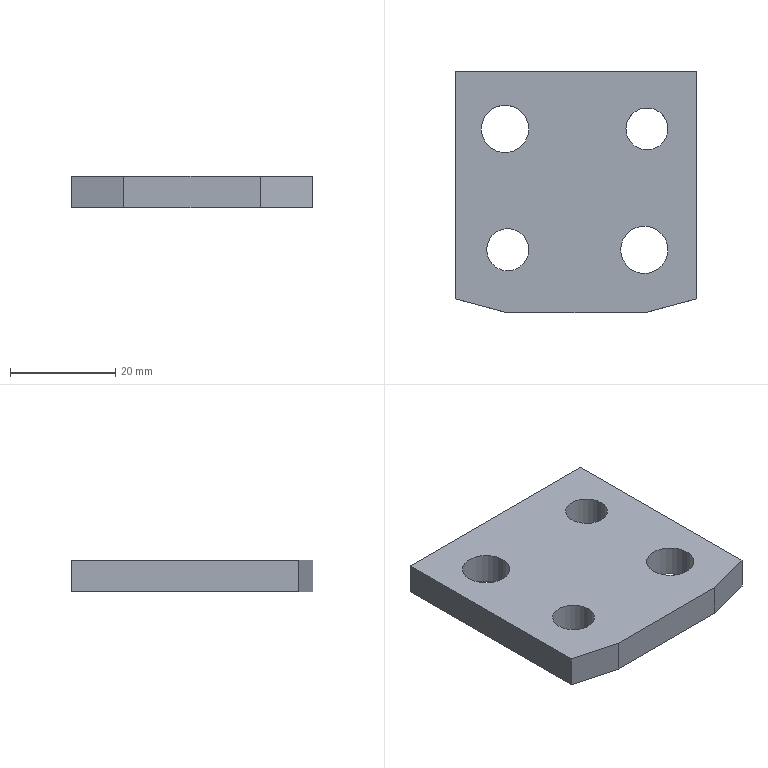Part | STEP file | gslz 2016.10.28-13_id682_x_t | 1 solid | 12 faces | box 46 x 46 x 6 mm | volume 11169 mm3 | plane 8 | cylinder 4 | commonest cylinder face diameters 8 x2 9 x2
STEP:
#1=CARTESIAN_POINT('',(0.,0.,0.));
#2=DIRECTION('',(0.,0.,1.));
#3=DIRECTION('',(1.,0.,0.));
#4=AXIS2_PLACEMENT_3D('',#1,#2,#3);
#5=CARTESIAN_POINT('',(1187.998,279.75,6.));
#6=VERTEX_POINT('',#5);
#7=CARTESIAN_POINT('',(1179.998,279.75,6.));
#8=VERTEX_POINT('',#7);
#9=CARTESIAN_POINT('',(1183.998,279.75,6.));
#10=DIRECTION('',(0.,0.,1.));
#11=DIRECTION('',(-1.,0.,0.));
#12=AXIS2_PLACEMENT_3D('',#9,#10,#11);
#13=CIRCLE('',#12,4.);
#14=CARTESIAN_POINT('',(1183.998,279.75,-73.));
#15=DIRECTION('',(0.,0.,1.));
#16=DIRECTION('',(1.,0.,0.));
#17=AXIS2_PLACEMENT_3D('',#14,#15,#16);
#18=CYLINDRICAL_SURFACE('',#17,4.);
#19=CARTESIAN_POINT('',(-3.142,79.));
#20=DIRECTION('',(1.,0.));
#21=VECTOR('',#20,1.);
#22=LINE('',#19,#21);
#23=(GEOMETRIC_REPRESENTATION_CONTEXT(2)PARAMETRIC_REPRESENTATION_CONTEXT()REPRESENTATION_CONTEXT('',''));
#24=DEFINITIONAL_REPRESENTATION('',(#22),#23);
#25=PCURVE('',#18,#24);
#26=CARTESIAN_POINT('',(1116.998,263.25,6.));
#27=DIRECTION('',(0.,0.,-1.));
#28=DIRECTION('',(-1.,0.,0.));
#29=AXIS2_PLACEMENT_3D('',#26,#27,#28);
#30=PLANE('',#29);
#31=CARTESIAN_POINT('',(-63.,16.5));
#32=CARTESIAN_POINT('',(-63.,9.572));
#33=CARTESIAN_POINT('',(-69.,13.036));
#34=CARTESIAN_POINT('',(-75.,16.5));
#35=CARTESIAN_POINT('',(-69.,19.964));
#36=CARTESIAN_POINT('',(-63.,23.428));
#37=CARTESIAN_POINT('',(-63.,16.5));
#38=(BOUNDED_CURVE()B_SPLINE_CURVE(2,(#31,#32,#33,#34,#35,#36,#37),.UNSPECIFIED.,.T.,.F.)B_SPLINE_CURVE_WITH_KNOTS((1,2,2,2,2,1),(-2.094,0.,2.094,4.189,6.283,8.378),.UNSPECIFIED.)CURVE()GEOMETRIC_REPRESENTATION_ITEM()RATIONAL_B_SPLINE_CURVE((1.,0.5,1.,0.5,1.,0.5,1.))REPRESENTATION_ITEM(''));
#39=(GEOMETRIC_REPRESENTATION_CONTEXT(2)PARAMETRIC_REPRESENTATION_CONTEXT()REPRESENTATION_CONTEXT('',''));
#40=DEFINITIONAL_REPRESENTATION('',(#38),#39);
#41=PCURVE('',#30,#40);
#42=SURFACE_CURVE('',#13,(#25,#41),.PCURVE_S1.);
#43=EDGE_CURVE('',#6,#8,#42,.T.);
#44=ORIENTED_EDGE('',*,*,#43,.F.);
#45=CARTESIAN_POINT('',(1187.998,279.75,0.));
#46=VERTEX_POINT('',#45);
#47=CARTESIAN_POINT('',(1187.998,279.75,0.));
#48=CARTESIAN_POINT('',(1187.998,279.75,6.));
#49=B_SPLINE_CURVE_WITH_KNOTS('',1,(#47,#48),.UNSPECIFIED.,.F.,.F.,(2,2),(73.,79.),.PIECEWISE_BEZIER_KNOTS.);
#50=CARTESIAN_POINT('',(0.,0.));
#51=DIRECTION('',(0.,1.));
#52=VECTOR('',#51,1.);
#53=LINE('',#50,#52);
#54=(GEOMETRIC_REPRESENTATION_CONTEXT(2)PARAMETRIC_REPRESENTATION_CONTEXT()REPRESENTATION_CONTEXT('',''));
#55=DEFINITIONAL_REPRESENTATION('',(#53),#54);
#56=PCURVE('',#18,#55);
#57=CARTESIAN_POINT('',(6.283,0.));
#58=DIRECTION('',(0.,1.));
#59=VECTOR('',#58,1.);
#60=LINE('',#57,#59);
#61=(GEOMETRIC_REPRESENTATION_CONTEXT(2)PARAMETRIC_REPRESENTATION_CONTEXT()REPRESENTATION_CONTEXT('',''));
#62=DEFINITIONAL_REPRESENTATION('',(#60),#61);
#63=PCURVE('',#18,#62);
#64=SEAM_CURVE('',#49,(#56,#63),.PCURVE_S1.);
#65=EDGE_CURVE('',#46,#6,#64,.T.);
#66=ORIENTED_EDGE('',*,*,#65,.F.);
#67=CARTESIAN_POINT('',(1183.998,279.75,0.));
#68=DIRECTION('',(0.,0.,-1.));
#69=DIRECTION('',(1.,0.,0.));
#70=AXIS2_PLACEMENT_3D('',#67,#68,#69);
#71=CIRCLE('',#70,4.);
#72=CARTESIAN_POINT('',(6.283,73.));
#73=DIRECTION('',(-1.,0.));
#74=VECTOR('',#73,1.);
#75=LINE('',#72,#74);
#76=(GEOMETRIC_REPRESENTATION_CONTEXT(2)PARAMETRIC_REPRESENTATION_CONTEXT()REPRESENTATION_CONTEXT('',''));
#77=DEFINITIONAL_REPRESENTATION('',(#75),#76);
#78=PCURVE('',#18,#77);
#79=CARTESIAN_POINT('',(1076.998,293.75,0.));
#80=DIRECTION('',(0.,0.,1.));
#81=DIRECTION('',(1.,0.,0.));
#82=AXIS2_PLACEMENT_3D('',#79,#80,#81);
#83=PLANE('',#82);
#84=CARTESIAN_POINT('',(111.,-14.));
#85=CARTESIAN_POINT('',(111.,-20.928));
#86=CARTESIAN_POINT('',(105.,-17.464));
#87=CARTESIAN_POINT('',(99.,-14.));
#88=CARTESIAN_POINT('',(105.,-10.536));
#89=CARTESIAN_POINT('',(111.,-7.072));
#90=CARTESIAN_POINT('',(111.,-14.));
#91=(BOUNDED_CURVE()B_SPLINE_CURVE(2,(#84,#85,#86,#87,#88,#89,#90),.UNSPECIFIED.,.T.,.F.)B_SPLINE_CURVE_WITH_KNOTS((1,2,2,2,2,1),(-2.094,0.,2.094,4.189,6.283,8.378),.UNSPECIFIED.)CURVE()GEOMETRIC_REPRESENTATION_ITEM()RATIONAL_B_SPLINE_CURVE((1.,0.5,1.,0.5,1.,0.5,1.))REPRESENTATION_ITEM(''));
#92=(GEOMETRIC_REPRESENTATION_CONTEXT(2)PARAMETRIC_REPRESENTATION_CONTEXT()REPRESENTATION_CONTEXT('',''));
#93=DEFINITIONAL_REPRESENTATION('',(#91),#92);
#94=PCURVE('',#83,#93);
#95=SURFACE_CURVE('',#71,(#78,#94),.PCURVE_S1.);
#96=EDGE_CURVE('',#46,#46,#95,.T.);
#97=ORIENTED_EDGE('',*,*,#96,.F.);
#98=ORIENTED_EDGE('',*,*,#65,.T.);
#99=CARTESIAN_POINT('',(1183.998,279.75,6.));
#100=DIRECTION('',(0.,0.,1.));
#101=DIRECTION('',(-1.,0.,0.));
#102=AXIS2_PLACEMENT_3D('',#99,#100,#101);
#103=CIRCLE('',#102,4.);
#104=CARTESIAN_POINT('',(3.142,79.));
#105=DIRECTION('',(1.,0.));
#106=VECTOR('',#105,1.);
#107=LINE('',#104,#106);
#108=(GEOMETRIC_REPRESENTATION_CONTEXT(2)PARAMETRIC_REPRESENTATION_CONTEXT()REPRESENTATION_CONTEXT('',''));
#109=DEFINITIONAL_REPRESENTATION('',(#107),#108);
#110=PCURVE('',#18,#109);
#111=CARTESIAN_POINT('',(-63.,16.5));
#112=CARTESIAN_POINT('',(-63.,9.572));
#113=CARTESIAN_POINT('',(-69.,13.036));
#114=CARTESIAN_POINT('',(-75.,16.5));
#115=CARTESIAN_POINT('',(-69.,19.964));
#116=CARTESIAN_POINT('',(-63.,23.428));
#117=CARTESIAN_POINT('',(-63.,16.5));
#118=(BOUNDED_CURVE()B_SPLINE_CURVE(2,(#111,#112,#113,#114,#115,#116,#117),.UNSPECIFIED.,.T.,.F.)B_SPLINE_CURVE_WITH_KNOTS((1,2,2,2,2,1),(-2.094,0.,2.094,4.189,6.283,8.378),.UNSPECIFIED.)CURVE()GEOMETRIC_REPRESENTATION_ITEM()RATIONAL_B_SPLINE_CURVE((1.,0.5,1.,0.5,1.,0.5,1.))REPRESENTATION_ITEM(''));
#119=(GEOMETRIC_REPRESENTATION_CONTEXT(2)PARAMETRIC_REPRESENTATION_CONTEXT()REPRESENTATION_CONTEXT('',''));
#120=DEFINITIONAL_REPRESENTATION('',(#118),#119);
#121=PCURVE('',#30,#120);
#122=SURFACE_CURVE('',#103,(#110,#121),.PCURVE_S1.);
#123=EDGE_CURVE('',#8,#6,#122,.T.);
#124=ORIENTED_EDGE('',*,*,#123,.F.);
#125=EDGE_LOOP('',(#44,#66,#97,#98,#124));
#126=FACE_BOUND('',#125,.F.);
#127=ADVANCED_FACE('',(#126),#18,.F.);
#128=CARTESIAN_POINT('',(1205.498,279.75,6.));
#129=VERTEX_POINT('',#128);
#130=CARTESIAN_POINT('',(1214.498,279.75,6.));
#131=VERTEX_POINT('',#130);
#132=CARTESIAN_POINT('',(1209.998,279.75,6.));
#133=DIRECTION('',(0.,0.,-1.));
#134=DIRECTION('',(-1.,0.,0.));
#135=AXIS2_PLACEMENT_3D('',#132,#133,#134);
#136=CIRCLE('',#135,4.5);
#137=CARTESIAN_POINT('',(1209.998,279.75,-73.));
#138=DIRECTION('',(0.,0.,1.));
#139=DIRECTION('',(1.,0.,0.));
#140=AXIS2_PLACEMENT_3D('',#137,#138,#139);
#141=CYLINDRICAL_SURFACE('',#140,4.5);
#142=CARTESIAN_POINT('',(3.142,79.));
#143=DIRECTION('',(-1.,0.));
#144=VECTOR('',#143,1.);
#145=LINE('',#142,#144);
#146=(GEOMETRIC_REPRESENTATION_CONTEXT(2)PARAMETRIC_REPRESENTATION_CONTEXT()REPRESENTATION_CONTEXT('',''));
#147=DEFINITIONAL_REPRESENTATION('',(#145),#146);
#148=PCURVE('',#141,#147);
#149=CARTESIAN_POINT('',(-93.,16.5));
#150=DIRECTION('',(1.,0.));
#151=AXIS2_PLACEMENT_2D('',#149,#150);
#152=CIRCLE('',#151,4.5);
#153=(GEOMETRIC_REPRESENTATION_CONTEXT(2)PARAMETRIC_REPRESENTATION_CONTEXT()REPRESENTATION_CONTEXT('',''));
#154=DEFINITIONAL_REPRESENTATION('',(#152),#153);
#155=PCURVE('',#30,#154);
#156=SURFACE_CURVE('',#136,(#148,#155),.PCURVE_S1.);
#157=EDGE_CURVE('',#129,#131,#156,.T.);
#158=ORIENTED_EDGE('',*,*,#157,.T.);
#159=CARTESIAN_POINT('',(1214.498,279.75,0.));
#160=VERTEX_POINT('',#159);
#161=CARTESIAN_POINT('',(1214.498,279.75,0.));
#162=CARTESIAN_POINT('',(1214.498,279.75,6.));
#163=B_SPLINE_CURVE_WITH_KNOTS('',1,(#161,#162),.UNSPECIFIED.,.F.,.F.,(2,2),(73.,79.),.PIECEWISE_BEZIER_KNOTS.);
#164=CARTESIAN_POINT('',(0.,0.));
#165=DIRECTION('',(0.,1.));
#166=VECTOR('',#165,1.);
#167=LINE('',#164,#166);
#168=(GEOMETRIC_REPRESENTATION_CONTEXT(2)PARAMETRIC_REPRESENTATION_CONTEXT()REPRESENTATION_CONTEXT('',''));
#169=DEFINITIONAL_REPRESENTATION('',(#167),#168);
#170=PCURVE('',#141,#169);
#171=CARTESIAN_POINT('',(6.283,0.));
#172=DIRECTION('',(0.,1.));
#173=VECTOR('',#172,1.);
#174=LINE('',#171,#173);
#175=(GEOMETRIC_REPRESENTATION_CONTEXT(2)PARAMETRIC_REPRESENTATION_CONTEXT()REPRESENTATION_CONTEXT('',''));
#176=DEFINITIONAL_REPRESENTATION('',(#174),#175);
#177=PCURVE('',#141,#176);
#178=SEAM_CURVE('',#163,(#170,#177),.PCURVE_S1.);
#179=EDGE_CURVE('',#160,#131,#178,.T.);
#180=ORIENTED_EDGE('',*,*,#179,.F.);
#181=CARTESIAN_POINT('',(1209.998,279.75,0.));
#182=DIRECTION('',(0.,0.,1.));
#183=DIRECTION('',(1.,0.,0.));
#184=AXIS2_PLACEMENT_3D('',#181,#182,#183);
#185=CIRCLE('',#184,4.5);
#186=CARTESIAN_POINT('',(0.,73.));
#187=DIRECTION('',(1.,0.));
#188=VECTOR('',#187,1.);
#189=LINE('',#186,#188);
#190=(GEOMETRIC_REPRESENTATION_CONTEXT(2)PARAMETRIC_REPRESENTATION_CONTEXT()REPRESENTATION_CONTEXT('',''));
#191=DEFINITIONAL_REPRESENTATION('',(#189),#190);
#192=PCURVE('',#141,#191);
#193=CARTESIAN_POINT('',(133.,-14.));
#194=DIRECTION('',(1.,0.));
#195=AXIS2_PLACEMENT_2D('',#193,#194);
#196=CIRCLE('',#195,4.5);
#197=(GEOMETRIC_REPRESENTATION_CONTEXT(2)PARAMETRIC_REPRESENTATION_CONTEXT()REPRESENTATION_CONTEXT('',''));
#198=DEFINITIONAL_REPRESENTATION('',(#196),#197);
#199=PCURVE('',#83,#198);
#200=SURFACE_CURVE('',#185,(#192,#199),.PCURVE_S1.);
#201=EDGE_CURVE('',#160,#160,#200,.T.);
#202=ORIENTED_EDGE('',*,*,#201,.T.);
#203=ORIENTED_EDGE('',*,*,#179,.T.);
#204=CARTESIAN_POINT('',(1209.998,279.75,6.));
#205=DIRECTION('',(0.,0.,-1.));
#206=DIRECTION('',(-1.,0.,0.));
#207=AXIS2_PLACEMENT_3D('',#204,#205,#206);
#208=CIRCLE('',#207,4.5);
#209=CARTESIAN_POINT('',(9.425,79.));
#210=DIRECTION('',(-1.,0.));
#211=VECTOR('',#210,1.);
#212=LINE('',#209,#211);
#213=(GEOMETRIC_REPRESENTATION_CONTEXT(2)PARAMETRIC_REPRESENTATION_CONTEXT()REPRESENTATION_CONTEXT('',''));
#214=DEFINITIONAL_REPRESENTATION('',(#212),#213);
#215=PCURVE('',#141,#214);
#216=CARTESIAN_POINT('',(-93.,16.5));
#217=DIRECTION('',(1.,0.));
#218=AXIS2_PLACEMENT_2D('',#216,#217);
#219=CIRCLE('',#218,4.5);
#220=(GEOMETRIC_REPRESENTATION_CONTEXT(2)PARAMETRIC_REPRESENTATION_CONTEXT()REPRESENTATION_CONTEXT('',''));
#221=DEFINITIONAL_REPRESENTATION('',(#219),#220);
#222=PCURVE('',#30,#221);
#223=SURFACE_CURVE('',#208,(#215,#222),.PCURVE_S1.);
#224=EDGE_CURVE('',#131,#129,#223,.T.);
#225=ORIENTED_EDGE('',*,*,#224,.T.);
#226=EDGE_LOOP('',(#158,#180,#202,#203,#225));
#227=FACE_BOUND('',#226,.F.);
#228=ADVANCED_FACE('',(#227),#141,.F.);
#229=CARTESIAN_POINT('',(1178.998,302.75,6.));
#230=VERTEX_POINT('',#229);
#231=CARTESIAN_POINT('',(1183.498,302.75,6.));
#232=DIRECTION('',(0.,0.,-1.));
#233=DIRECTION('',(-1.,0.,0.));
#234=AXIS2_PLACEMENT_3D('',#231,#232,#233);
#235=CIRCLE('',#234,4.5);
#236=CARTESIAN_POINT('',(1183.498,302.75,47.));
#237=DIRECTION('',(0.,0.,-1.));
#238=DIRECTION('',(-1.,0.,0.));
#239=AXIS2_PLACEMENT_3D('',#236,#237,#238);
#240=CYLINDRICAL_SURFACE('',#239,4.5);
#241=CARTESIAN_POINT('',(0.,41.));
#242=DIRECTION('',(1.,0.));
#243=VECTOR('',#242,1.);
#244=LINE('',#241,#243);
#245=(GEOMETRIC_REPRESENTATION_CONTEXT(2)PARAMETRIC_REPRESENTATION_CONTEXT()REPRESENTATION_CONTEXT('',''));
#246=DEFINITIONAL_REPRESENTATION('',(#244),#245);
#247=PCURVE('',#240,#246);
#248=CARTESIAN_POINT('',(-66.5,39.5));
#249=DIRECTION('',(1.,0.));
#250=AXIS2_PLACEMENT_2D('',#248,#249);
#251=CIRCLE('',#250,4.5);
#252=(GEOMETRIC_REPRESENTATION_CONTEXT(2)PARAMETRIC_REPRESENTATION_CONTEXT()REPRESENTATION_CONTEXT('',''));
#253=DEFINITIONAL_REPRESENTATION('',(#251),#252);
#254=PCURVE('',#30,#253);
#255=SURFACE_CURVE('',#235,(#247,#254),.PCURVE_S1.);
#256=EDGE_CURVE('',#230,#230,#255,.T.);
#257=ORIENTED_EDGE('',*,*,#256,.T.);
#258=CARTESIAN_POINT('',(1178.998,302.75,0.));
#259=VERTEX_POINT('',#258);
#260=CARTESIAN_POINT('',(1178.998,302.75,6.));
#261=CARTESIAN_POINT('',(1178.998,302.75,0.));
#262=B_SPLINE_CURVE_WITH_KNOTS('',1,(#260,#261),.UNSPECIFIED.,.F.,.F.,(2,2),(41.,47.),.PIECEWISE_BEZIER_KNOTS.);
#263=CARTESIAN_POINT('',(6.283,0.));
#264=DIRECTION('',(0.,1.));
#265=VECTOR('',#264,1.);
#266=LINE('',#263,#265);
#267=(GEOMETRIC_REPRESENTATION_CONTEXT(2)PARAMETRIC_REPRESENTATION_CONTEXT()REPRESENTATION_CONTEXT('',''));
#268=DEFINITIONAL_REPRESENTATION('',(#266),#267);
#269=PCURVE('',#240,#268);
#270=CARTESIAN_POINT('',(0.,0.));
#271=DIRECTION('',(0.,1.));
#272=VECTOR('',#271,1.);
#273=LINE('',#270,#272);
#274=(GEOMETRIC_REPRESENTATION_CONTEXT(2)PARAMETRIC_REPRESENTATION_CONTEXT()REPRESENTATION_CONTEXT('',''));
#275=DEFINITIONAL_REPRESENTATION('',(#273),#274);
#276=PCURVE('',#240,#275);
#277=SEAM_CURVE('',#262,(#269,#276),.PCURVE_S1.);
#278=EDGE_CURVE('',#230,#259,#277,.T.);
#279=ORIENTED_EDGE('',*,*,#278,.T.);
#280=CARTESIAN_POINT('',(1187.998,302.75,0.));
#281=VERTEX_POINT('',#280);
#282=CARTESIAN_POINT('',(1183.498,302.75,0.));
#283=DIRECTION('',(0.,0.,1.));
#284=DIRECTION('',(1.,0.,0.));
#285=AXIS2_PLACEMENT_3D('',#282,#283,#284);
#286=CIRCLE('',#285,4.5);
#287=CARTESIAN_POINT('',(9.425,47.));
#288=DIRECTION('',(-1.,0.));
#289=VECTOR('',#288,1.);
#290=LINE('',#287,#289);
#291=(GEOMETRIC_REPRESENTATION_CONTEXT(2)PARAMETRIC_REPRESENTATION_CONTEXT()REPRESENTATION_CONTEXT('',''));
#292=DEFINITIONAL_REPRESENTATION('',(#290),#291);
#293=PCURVE('',#240,#292);
#294=CARTESIAN_POINT('',(106.5,9.));
#295=DIRECTION('',(1.,0.));
#296=AXIS2_PLACEMENT_2D('',#294,#295);
#297=CIRCLE('',#296,4.5);
#298=(GEOMETRIC_REPRESENTATION_CONTEXT(2)PARAMETRIC_REPRESENTATION_CONTEXT()REPRESENTATION_CONTEXT('',''));
#299=DEFINITIONAL_REPRESENTATION('',(#297),#298);
#300=PCURVE('',#83,#299);
#301=SURFACE_CURVE('',#286,(#293,#300),.PCURVE_S1.);
#302=EDGE_CURVE('',#259,#281,#301,.T.);
#303=ORIENTED_EDGE('',*,*,#302,.T.);
#304=CARTESIAN_POINT('',(1183.498,302.75,0.));
#305=DIRECTION('',(0.,0.,1.));
#306=DIRECTION('',(1.,0.,0.));
#307=AXIS2_PLACEMENT_3D('',#304,#305,#306);
#308=CIRCLE('',#307,4.5);
#309=CARTESIAN_POINT('',(3.142,47.));
#310=DIRECTION('',(-1.,0.));
#311=VECTOR('',#310,1.);
#312=LINE('',#309,#311);
#313=(GEOMETRIC_REPRESENTATION_CONTEXT(2)PARAMETRIC_REPRESENTATION_CONTEXT()REPRESENTATION_CONTEXT('',''));
#314=DEFINITIONAL_REPRESENTATION('',(#312),#313);
#315=PCURVE('',#240,#314);
#316=CARTESIAN_POINT('',(106.5,9.));
#317=DIRECTION('',(1.,0.));
#318=AXIS2_PLACEMENT_2D('',#316,#317);
#319=CIRCLE('',#318,4.5);
#320=(GEOMETRIC_REPRESENTATION_CONTEXT(2)PARAMETRIC_REPRESENTATION_CONTEXT()REPRESENTATION_CONTEXT('',''));
#321=DEFINITIONAL_REPRESENTATION('',(#319),#320);
#322=PCURVE('',#83,#321);
#323=SURFACE_CURVE('',#308,(#315,#322),.PCURVE_S1.);
#324=EDGE_CURVE('',#281,#259,#323,.T.);
#325=ORIENTED_EDGE('',*,*,#324,.T.);
#326=ORIENTED_EDGE('',*,*,#278,.F.);
#327=EDGE_LOOP('',(#257,#279,#303,#325,#326));
#328=FACE_BOUND('',#327,.F.);
#329=ADVANCED_FACE('',(#328),#240,.F.);
#330=CARTESIAN_POINT('',(1209.999,267.75,0.));
#331=VERTEX_POINT('',#330);
#332=CARTESIAN_POINT('',(1209.999,267.75,6.));
#333=VERTEX_POINT('',#332);
#334=CARTESIAN_POINT('',(1209.999,267.75,8.));
#335=DIRECTION('',(0.,0.,1.));
#336=VECTOR('',#335,1.);
#337=LINE('',#334,#336);
#338=CARTESIAN_POINT('',(1087.,267.75,8.));
#339=DIRECTION('',(0.,1.,0.));
#340=DIRECTION('',(0.,0.,1.));
#341=AXIS2_PLACEMENT_3D('',#338,#339,#340);
#342=PLANE('',#341);
#343=CARTESIAN_POINT('',(0.,122.999));
#344=DIRECTION('',(1.,0.));
#345=VECTOR('',#344,1.);
#346=LINE('',#343,#345);
#347=(GEOMETRIC_REPRESENTATION_CONTEXT(2)PARAMETRIC_REPRESENTATION_CONTEXT()REPRESENTATION_CONTEXT('',''));
#348=DEFINITIONAL_REPRESENTATION('',(#346),#347);
#349=PCURVE('',#342,#348);
#350=CARTESIAN_POINT('',(1209.999,267.75,8.));
#351=DIRECTION('',(-0.2588,0.9659,0.));
#352=DIRECTION('',(-0.9659,-0.2588,0.));
#353=AXIS2_PLACEMENT_3D('',#350,#351,#352);
#354=PLANE('',#353);
#355=CARTESIAN_POINT('',(0.,0.));
#356=DIRECTION('',(0.,1.));
#357=VECTOR('',#356,1.);
#358=LINE('',#355,#357);
#359=(GEOMETRIC_REPRESENTATION_CONTEXT(2)PARAMETRIC_REPRESENTATION_CONTEXT()REPRESENTATION_CONTEXT('',''));
#360=DEFINITIONAL_REPRESENTATION('',(#358),#359);
#361=PCURVE('',#354,#360);
#362=SURFACE_CURVE('',#337,(#349,#361),.PCURVE_S1.);
#363=EDGE_CURVE('',#331,#333,#362,.T.);
#364=ORIENTED_EDGE('',*,*,#363,.T.);
#365=CARTESIAN_POINT('',(1184.,267.75,6.));
#366=VERTEX_POINT('',#365);
#367=CARTESIAN_POINT('',(1087.,267.75,6.));
#368=DIRECTION('',(-1.,0.,0.));
#369=VECTOR('',#368,1.);
#370=LINE('',#367,#369);
#371=CARTESIAN_POINT('',(-2.,0.));
#372=DIRECTION('',(0.,-1.));
#373=VECTOR('',#372,1.);
#374=LINE('',#371,#373);
#375=(GEOMETRIC_REPRESENTATION_CONTEXT(2)PARAMETRIC_REPRESENTATION_CONTEXT()REPRESENTATION_CONTEXT('',''));
#376=DEFINITIONAL_REPRESENTATION('',(#374),#375);
#377=PCURVE('',#342,#376);
#378=CARTESIAN_POINT('',(29.998,4.5));
#379=DIRECTION('',(1.,0.));
#380=VECTOR('',#379,1.);
#381=LINE('',#378,#380);
#382=(GEOMETRIC_REPRESENTATION_CONTEXT(2)PARAMETRIC_REPRESENTATION_CONTEXT()REPRESENTATION_CONTEXT('',''));
#383=DEFINITIONAL_REPRESENTATION('',(#381),#382);
#384=PCURVE('',#30,#383);
#385=SURFACE_CURVE('',#370,(#377,#384),.PCURVE_S1.);
#386=EDGE_CURVE('',#333,#366,#385,.T.);
#387=ORIENTED_EDGE('',*,*,#386,.T.);
#388=CARTESIAN_POINT('',(1184.,267.75,0.));
#389=VERTEX_POINT('',#388);
#390=CARTESIAN_POINT('',(1184.,267.75,8.));
#391=DIRECTION('',(0.,0.,1.));
#392=VECTOR('',#391,1.);
#393=LINE('',#390,#392);
#394=CARTESIAN_POINT('',(0.,97.));
#395=DIRECTION('',(1.,0.));
#396=VECTOR('',#395,1.);
#397=LINE('',#394,#396);
#398=(GEOMETRIC_REPRESENTATION_CONTEXT(2)PARAMETRIC_REPRESENTATION_CONTEXT()REPRESENTATION_CONTEXT('',''));
#399=DEFINITIONAL_REPRESENTATION('',(#397),#398);
#400=PCURVE('',#342,#399);
#401=CARTESIAN_POINT('',(1173.998,270.43,8.));
#402=DIRECTION('',(0.2588,0.9659,0.));
#403=DIRECTION('',(-0.9659,0.2588,0.));
#404=AXIS2_PLACEMENT_3D('',#401,#402,#403);
#405=PLANE('',#404);
#406=CARTESIAN_POINT('',(-10.355,0.));
#407=DIRECTION('',(0.,1.));
#408=VECTOR('',#407,1.);
#409=LINE('',#406,#408);
#410=(GEOMETRIC_REPRESENTATION_CONTEXT(2)PARAMETRIC_REPRESENTATION_CONTEXT()REPRESENTATION_CONTEXT('',''));
#411=DEFINITIONAL_REPRESENTATION('',(#409),#410);
#412=PCURVE('',#405,#411);
#413=SURFACE_CURVE('',#393,(#400,#412),.PCURVE_S1.);
#414=EDGE_CURVE('',#389,#366,#413,.T.);
#415=ORIENTED_EDGE('',*,*,#414,.F.);
#416=CARTESIAN_POINT('',(1087.,267.75,0.));
#417=DIRECTION('',(1.,0.,0.));
#418=VECTOR('',#417,1.);
#419=LINE('',#416,#418);
#420=CARTESIAN_POINT('',(-8.,0.));
#421=DIRECTION('',(0.,1.));
#422=VECTOR('',#421,1.);
#423=LINE('',#420,#422);
#424=(GEOMETRIC_REPRESENTATION_CONTEXT(2)PARAMETRIC_REPRESENTATION_CONTEXT()REPRESENTATION_CONTEXT('',''));
#425=DEFINITIONAL_REPRESENTATION('',(#423),#424);
#426=PCURVE('',#342,#425);
#427=CARTESIAN_POINT('',(10.002,-26.));
#428=DIRECTION('',(1.,0.));
#429=VECTOR('',#428,1.);
#430=LINE('',#427,#429);
#431=(GEOMETRIC_REPRESENTATION_CONTEXT(2)PARAMETRIC_REPRESENTATION_CONTEXT()REPRESENTATION_CONTEXT('',''));
#432=DEFINITIONAL_REPRESENTATION('',(#430),#431);
#433=PCURVE('',#83,#432);
#434=SURFACE_CURVE('',#419,(#426,#433),.PCURVE_S1.);
#435=EDGE_CURVE('',#389,#331,#434,.T.);
#436=ORIENTED_EDGE('',*,*,#435,.T.);
#437=EDGE_LOOP('',(#364,#387,#415,#436));
#438=FACE_BOUND('',#437,.T.);
#439=ADVANCED_FACE('',(#438),#342,.F.);
#440=CARTESIAN_POINT('',(1219.998,270.429,6.));
#441=VERTEX_POINT('',#440);
#442=CARTESIAN_POINT('',(1219.998,270.429,0.));
#443=VERTEX_POINT('',#442);
#444=CARTESIAN_POINT('',(1219.998,270.429,8.));
#445=DIRECTION('',(0.,0.,-1.));
#446=VECTOR('',#445,1.);
#447=LINE('',#444,#446);
#448=CARTESIAN_POINT('',(-10.352,0.));
#449=DIRECTION('',(0.,-1.));
#450=VECTOR('',#449,1.);
#451=LINE('',#448,#450);
#452=(GEOMETRIC_REPRESENTATION_CONTEXT(2)PARAMETRIC_REPRESENTATION_CONTEXT()REPRESENTATION_CONTEXT('',''));
#453=DEFINITIONAL_REPRESENTATION('',(#451),#452);
#454=PCURVE('',#354,#453);
#455=CARTESIAN_POINT('',(1219.998,260.75,16.));
#456=DIRECTION('',(-1.,0.,0.));
#457=DIRECTION('',(0.,0.,1.));
#458=AXIS2_PLACEMENT_3D('',#455,#456,#457);
#459=PLANE('',#458);
#460=CARTESIAN_POINT('',(-8.,9.679));
#461=DIRECTION('',(-1.,0.));
#462=VECTOR('',#461,1.);
#463=LINE('',#460,#462);
#464=(GEOMETRIC_REPRESENTATION_CONTEXT(2)PARAMETRIC_REPRESENTATION_CONTEXT()REPRESENTATION_CONTEXT('',''));
#465=DEFINITIONAL_REPRESENTATION('',(#463),#464);
#466=PCURVE('',#459,#465);
#467=SURFACE_CURVE('',#447,(#454,#466),.PCURVE_S1.);
#468=EDGE_CURVE('',#441,#443,#467,.T.);
#469=ORIENTED_EDGE('',*,*,#468,.F.);
#470=CARTESIAN_POINT('',(1209.999,267.75,6.));
#471=DIRECTION('',(-0.9659,-0.2588,0.));
#472=VECTOR('',#471,1.);
#473=LINE('',#470,#472);
#474=CARTESIAN_POINT('',(0.,-2.));
#475=DIRECTION('',(1.,0.));
#476=VECTOR('',#475,1.);
#477=LINE('',#474,#476);
#478=(GEOMETRIC_REPRESENTATION_CONTEXT(2)PARAMETRIC_REPRESENTATION_CONTEXT()REPRESENTATION_CONTEXT('',''));
#479=DEFINITIONAL_REPRESENTATION('',(#477),#478);
#480=PCURVE('',#354,#479);
#481=CARTESIAN_POINT('',(-93.001,4.5));
#482=DIRECTION('',(0.9659,-0.2588));
#483=VECTOR('',#482,1.);
#484=LINE('',#481,#483);
#485=(GEOMETRIC_REPRESENTATION_CONTEXT(2)PARAMETRIC_REPRESENTATION_CONTEXT()REPRESENTATION_CONTEXT('',''));
#486=DEFINITIONAL_REPRESENTATION('',(#484),#485);
#487=PCURVE('',#30,#486);
#488=SURFACE_CURVE('',#473,(#480,#487),.PCURVE_S1.);
#489=EDGE_CURVE('',#441,#333,#488,.T.);
#490=ORIENTED_EDGE('',*,*,#489,.T.);
#491=ORIENTED_EDGE('',*,*,#363,.F.);
#492=CARTESIAN_POINT('',(1209.999,267.75,0.));
#493=DIRECTION('',(0.9659,0.2588,0.));
#494=VECTOR('',#493,1.);
#495=LINE('',#492,#494);
#496=CARTESIAN_POINT('',(0.,-8.));
#497=DIRECTION('',(-1.,0.));
#498=VECTOR('',#497,1.);
#499=LINE('',#496,#498);
#500=(GEOMETRIC_REPRESENTATION_CONTEXT(2)PARAMETRIC_REPRESENTATION_CONTEXT()REPRESENTATION_CONTEXT('',''));
#501=DEFINITIONAL_REPRESENTATION('',(#499),#500);
#502=PCURVE('',#354,#501);
#503=CARTESIAN_POINT('',(133.001,-26.));
#504=DIRECTION('',(0.9659,0.2588));
#505=VECTOR('',#504,1.);
#506=LINE('',#503,#505);
#507=(GEOMETRIC_REPRESENTATION_CONTEXT(2)PARAMETRIC_REPRESENTATION_CONTEXT()REPRESENTATION_CONTEXT('',''));
#508=DEFINITIONAL_REPRESENTATION('',(#506),#507);
#509=PCURVE('',#83,#508);
#510=SURFACE_CURVE('',#495,(#502,#509),.PCURVE_S1.);
#511=EDGE_CURVE('',#331,#443,#510,.T.);
#512=ORIENTED_EDGE('',*,*,#511,.T.);
#513=EDGE_LOOP('',(#469,#490,#491,#512));
#514=FACE_BOUND('',#513,.T.);
#515=ADVANCED_FACE('',(#514),#354,.F.);
#516=CARTESIAN_POINT('',(1219.998,313.75,6.));
#517=VERTEX_POINT('',#516);
#518=CARTESIAN_POINT('',(1219.998,313.75,0.));
#519=VERTEX_POINT('',#518);
#520=CARTESIAN_POINT('',(1219.998,313.75,16.));
#521=DIRECTION('',(0.,0.,-1.));
#522=VECTOR('',#521,1.);
#523=LINE('',#520,#522);
#524=CARTESIAN_POINT('',(0.,53.));
#525=DIRECTION('',(-1.,0.));
#526=VECTOR('',#525,1.);
#527=LINE('',#524,#526);
#528=(GEOMETRIC_REPRESENTATION_CONTEXT(2)PARAMETRIC_REPRESENTATION_CONTEXT()REPRESENTATION_CONTEXT('',''));
#529=DEFINITIONAL_REPRESENTATION('',(#527),#528);
#530=PCURVE('',#459,#529);
#531=CARTESIAN_POINT('',(1156.998,313.75,16.));
#532=DIRECTION('',(0.,-1.,0.));
#533=DIRECTION('',(0.,0.,-1.));
#534=AXIS2_PLACEMENT_3D('',#531,#532,#533);
#535=PLANE('',#534);
#536=CARTESIAN_POINT('',(0.,63.));
#537=DIRECTION('',(1.,0.));
#538=VECTOR('',#537,1.);
#539=LINE('',#536,#538);
#540=(GEOMETRIC_REPRESENTATION_CONTEXT(2)PARAMETRIC_REPRESENTATION_CONTEXT()REPRESENTATION_CONTEXT('',''));
#541=DEFINITIONAL_REPRESENTATION('',(#539),#540);
#542=PCURVE('',#535,#541);
#543=SURFACE_CURVE('',#523,(#530,#542),.PCURVE_S1.);
#544=EDGE_CURVE('',#517,#519,#543,.T.);
#545=ORIENTED_EDGE('',*,*,#544,.F.);
#546=CARTESIAN_POINT('',(1219.998,260.75,6.));
#547=DIRECTION('',(0.,-1.,0.));
#548=VECTOR('',#547,1.);
#549=LINE('',#546,#548);
#550=CARTESIAN_POINT('',(-10.,0.));
#551=DIRECTION('',(0.,-1.));
#552=VECTOR('',#551,1.);
#553=LINE('',#550,#552);
#554=(GEOMETRIC_REPRESENTATION_CONTEXT(2)PARAMETRIC_REPRESENTATION_CONTEXT()REPRESENTATION_CONTEXT('',''));
#555=DEFINITIONAL_REPRESENTATION('',(#553),#554);
#556=PCURVE('',#459,#555);
#557=CARTESIAN_POINT('',(-103.,-2.5));
#558=DIRECTION('',(0.,-1.));
#559=VECTOR('',#558,1.);
#560=LINE('',#557,#559);
#561=(GEOMETRIC_REPRESENTATION_CONTEXT(2)PARAMETRIC_REPRESENTATION_CONTEXT()REPRESENTATION_CONTEXT('',''));
#562=DEFINITIONAL_REPRESENTATION('',(#560),#561);
#563=PCURVE('',#30,#562);
#564=SURFACE_CURVE('',#549,(#556,#563),.PCURVE_S1.);
#565=EDGE_CURVE('',#517,#441,#564,.T.);
#566=ORIENTED_EDGE('',*,*,#565,.T.);
#567=ORIENTED_EDGE('',*,*,#468,.T.);
#568=CARTESIAN_POINT('',(1219.998,260.75,0.));
#569=DIRECTION('',(0.,1.,0.));
#570=VECTOR('',#569,1.);
#571=LINE('',#568,#570);
#572=CARTESIAN_POINT('',(-16.,0.));
#573=DIRECTION('',(0.,1.));
#574=VECTOR('',#573,1.);
#575=LINE('',#572,#574);
#576=(GEOMETRIC_REPRESENTATION_CONTEXT(2)PARAMETRIC_REPRESENTATION_CONTEXT()REPRESENTATION_CONTEXT('',''));
#577=DEFINITIONAL_REPRESENTATION('',(#575),#576);
#578=PCURVE('',#459,#577);
#579=CARTESIAN_POINT('',(143.,-33.));
#580=DIRECTION('',(0.,1.));
#581=VECTOR('',#580,1.);
#582=LINE('',#579,#581);
#583=(GEOMETRIC_REPRESENTATION_CONTEXT(2)PARAMETRIC_REPRESENTATION_CONTEXT()REPRESENTATION_CONTEXT('',''));
#584=DEFINITIONAL_REPRESENTATION('',(#582),#583);
#585=PCURVE('',#83,#584);
#586=SURFACE_CURVE('',#571,(#578,#585),.PCURVE_S1.);
#587=EDGE_CURVE('',#443,#519,#586,.T.);
#588=ORIENTED_EDGE('',*,*,#587,.T.);
#589=EDGE_LOOP('',(#545,#566,#567,#588));
#590=FACE_BOUND('',#589,.T.);
#591=ADVANCED_FACE('',(#590),#459,.F.);
#592=CARTESIAN_POINT('',(1173.998,313.75,6.));
#593=VERTEX_POINT('',#592);
#594=CARTESIAN_POINT('',(1173.998,313.75,0.));
#595=VERTEX_POINT('',#594);
#596=CARTESIAN_POINT('',(1173.998,313.75,16.));
#597=DIRECTION('',(0.,0.,-1.));
#598=VECTOR('',#597,1.);
#599=LINE('',#596,#598);
#600=CARTESIAN_POINT('',(0.,17.));
#601=DIRECTION('',(1.,0.));
#602=VECTOR('',#601,1.);
#603=LINE('',#600,#602);
#604=(GEOMETRIC_REPRESENTATION_CONTEXT(2)PARAMETRIC_REPRESENTATION_CONTEXT()REPRESENTATION_CONTEXT('',''));
#605=DEFINITIONAL_REPRESENTATION('',(#603),#604);
#606=PCURVE('',#535,#605);
#607=CARTESIAN_POINT('',(1173.998,293.75,16.));
#608=DIRECTION('',(1.,0.,0.));
#609=DIRECTION('',(0.,0.,-1.));
#610=AXIS2_PLACEMENT_3D('',#607,#608,#609);
#611=PLANE('',#610);
#612=CARTESIAN_POINT('',(0.,20.));
#613=DIRECTION('',(1.,0.));
#614=VECTOR('',#613,1.);
#615=LINE('',#612,#614);
#616=(GEOMETRIC_REPRESENTATION_CONTEXT(2)PARAMETRIC_REPRESENTATION_CONTEXT()REPRESENTATION_CONTEXT('',''));
#617=DEFINITIONAL_REPRESENTATION('',(#615),#616);
#618=PCURVE('',#611,#617);
#619=SURFACE_CURVE('',#599,(#606,#618),.PCURVE_S1.);
#620=EDGE_CURVE('',#593,#595,#619,.T.);
#621=ORIENTED_EDGE('',*,*,#620,.F.);
#622=CARTESIAN_POINT('',(1156.998,313.75,6.));
#623=DIRECTION('',(1.,0.,0.));
#624=VECTOR('',#623,1.);
#625=LINE('',#622,#624);
#626=CARTESIAN_POINT('',(10.,0.));
#627=DIRECTION('',(0.,1.));
#628=VECTOR('',#627,1.);
#629=LINE('',#626,#628);
#630=(GEOMETRIC_REPRESENTATION_CONTEXT(2)PARAMETRIC_REPRESENTATION_CONTEXT()REPRESENTATION_CONTEXT('',''));
#631=DEFINITIONAL_REPRESENTATION('',(#629),#630);
#632=PCURVE('',#535,#631);
#633=CARTESIAN_POINT('',(-40.,50.5));
#634=DIRECTION('',(-1.,0.));
#635=VECTOR('',#634,1.);
#636=LINE('',#633,#635);
#637=(GEOMETRIC_REPRESENTATION_CONTEXT(2)PARAMETRIC_REPRESENTATION_CONTEXT()REPRESENTATION_CONTEXT('',''));
#638=DEFINITIONAL_REPRESENTATION('',(#636),#637);
#639=PCURVE('',#30,#638);
#640=SURFACE_CURVE('',#625,(#632,#639),.PCURVE_S1.);
#641=EDGE_CURVE('',#593,#517,#640,.T.);
#642=ORIENTED_EDGE('',*,*,#641,.T.);
#643=ORIENTED_EDGE('',*,*,#544,.T.);
#644=CARTESIAN_POINT('',(1156.998,313.75,0.));
#645=DIRECTION('',(-1.,0.,0.));
#646=VECTOR('',#645,1.);
#647=LINE('',#644,#646);
#648=CARTESIAN_POINT('',(16.,0.));
#649=DIRECTION('',(0.,-1.));
#650=VECTOR('',#649,1.);
#651=LINE('',#648,#650);
#652=(GEOMETRIC_REPRESENTATION_CONTEXT(2)PARAMETRIC_REPRESENTATION_CONTEXT()REPRESENTATION_CONTEXT('',''));
#653=DEFINITIONAL_REPRESENTATION('',(#651),#652);
#654=PCURVE('',#535,#653);
#655=CARTESIAN_POINT('',(80.,20.));
#656=DIRECTION('',(-1.,0.));
#657=VECTOR('',#656,1.);
#658=LINE('',#655,#657);
#659=(GEOMETRIC_REPRESENTATION_CONTEXT(2)PARAMETRIC_REPRESENTATION_CONTEXT()REPRESENTATION_CONTEXT('',''));
#660=DEFINITIONAL_REPRESENTATION('',(#658),#659);
#661=PCURVE('',#83,#660);
#662=SURFACE_CURVE('',#647,(#654,#661),.PCURVE_S1.);
#663=EDGE_CURVE('',#519,#595,#662,.T.);
#664=ORIENTED_EDGE('',*,*,#663,.T.);
#665=EDGE_LOOP('',(#621,#642,#643,#664));
#666=FACE_BOUND('',#665,.T.);
#667=ADVANCED_FACE('',(#666),#535,.F.);
#668=CARTESIAN_POINT('',(1173.998,270.43,6.));
#669=VERTEX_POINT('',#668);
#670=CARTESIAN_POINT('',(1173.998,270.43,0.));
#671=VERTEX_POINT('',#670);
#672=CARTESIAN_POINT('',(1173.998,270.43,8.));
#673=DIRECTION('',(0.,0.,-1.));
#674=VECTOR('',#673,1.);
#675=LINE('',#672,#674);
#676=CARTESIAN_POINT('',(8.,-23.32));
#677=DIRECTION('',(1.,0.));
#678=VECTOR('',#677,1.);
#679=LINE('',#676,#678);
#680=(GEOMETRIC_REPRESENTATION_CONTEXT(2)PARAMETRIC_REPRESENTATION_CONTEXT()REPRESENTATION_CONTEXT('',''));
#681=DEFINITIONAL_REPRESENTATION('',(#679),#680);
#682=PCURVE('',#611,#681);
#683=CARTESIAN_POINT('',(0.,0.));
#684=DIRECTION('',(0.,-1.));
#685=VECTOR('',#684,1.);
#686=LINE('',#683,#685);
#687=(GEOMETRIC_REPRESENTATION_CONTEXT(2)PARAMETRIC_REPRESENTATION_CONTEXT()REPRESENTATION_CONTEXT('',''));
#688=DEFINITIONAL_REPRESENTATION('',(#686),#687);
#689=PCURVE('',#405,#688);
#690=SURFACE_CURVE('',#675,(#682,#689),.PCURVE_S1.);
#691=EDGE_CURVE('',#669,#671,#690,.T.);
#692=ORIENTED_EDGE('',*,*,#691,.F.);
#693=CARTESIAN_POINT('',(1173.998,293.75,6.));
#694=DIRECTION('',(0.,1.,0.));
#695=VECTOR('',#694,1.);
#696=LINE('',#693,#695);
#697=CARTESIAN_POINT('',(10.,0.));
#698=DIRECTION('',(0.,1.));
#699=VECTOR('',#698,1.);
#700=LINE('',#697,#699);
#701=(GEOMETRIC_REPRESENTATION_CONTEXT(2)PARAMETRIC_REPRESENTATION_CONTEXT()REPRESENTATION_CONTEXT('',''));
#702=DEFINITIONAL_REPRESENTATION('',(#700),#701);
#703=PCURVE('',#611,#702);
#704=CARTESIAN_POINT('',(-57.,30.5));
#705=DIRECTION('',(0.,1.));
#706=VECTOR('',#705,1.);
#707=LINE('',#704,#706);
#708=(GEOMETRIC_REPRESENTATION_CONTEXT(2)PARAMETRIC_REPRESENTATION_CONTEXT()REPRESENTATION_CONTEXT('',''));
#709=DEFINITIONAL_REPRESENTATION('',(#707),#708);
#710=PCURVE('',#30,#709);
#711=SURFACE_CURVE('',#696,(#703,#710),.PCURVE_S1.);
#712=EDGE_CURVE('',#669,#593,#711,.T.);
#713=ORIENTED_EDGE('',*,*,#712,.T.);
#714=ORIENTED_EDGE('',*,*,#620,.T.);
#715=CARTESIAN_POINT('',(1173.998,293.75,0.));
#716=DIRECTION('',(0.,-1.,0.));
#717=VECTOR('',#716,1.);
#718=LINE('',#715,#717);
#719=CARTESIAN_POINT('',(16.,0.));
#720=DIRECTION('',(0.,-1.));
#721=VECTOR('',#720,1.);
#722=LINE('',#719,#721);
#723=(GEOMETRIC_REPRESENTATION_CONTEXT(2)PARAMETRIC_REPRESENTATION_CONTEXT()REPRESENTATION_CONTEXT('',''));
#724=DEFINITIONAL_REPRESENTATION('',(#722),#723);
#725=PCURVE('',#611,#724);
#726=CARTESIAN_POINT('',(97.,0.));
#727=DIRECTION('',(0.,-1.));
#728=VECTOR('',#727,1.);
#729=LINE('',#726,#728);
#730=(GEOMETRIC_REPRESENTATION_CONTEXT(2)PARAMETRIC_REPRESENTATION_CONTEXT()REPRESENTATION_CONTEXT('',''));
#731=DEFINITIONAL_REPRESENTATION('',(#729),#730);
#732=PCURVE('',#83,#731);
#733=SURFACE_CURVE('',#718,(#725,#732),.PCURVE_S1.);
#734=EDGE_CURVE('',#595,#671,#733,.T.);
#735=ORIENTED_EDGE('',*,*,#734,.T.);
#736=EDGE_LOOP('',(#692,#713,#714,#735));
#737=FACE_BOUND('',#736,.T.);
#738=ADVANCED_FACE('',(#737),#611,.F.);
#739=ORIENTED_EDGE('',*,*,#414,.T.);
#740=CARTESIAN_POINT('',(1173.998,270.43,6.));
#741=DIRECTION('',(-0.9659,0.2588,0.));
#742=VECTOR('',#741,1.);
#743=LINE('',#740,#742);
#744=CARTESIAN_POINT('',(0.,-2.));
#745=DIRECTION('',(1.,0.));
#746=VECTOR('',#745,1.);
#747=LINE('',#744,#746);
#748=(GEOMETRIC_REPRESENTATION_CONTEXT(2)PARAMETRIC_REPRESENTATION_CONTEXT()REPRESENTATION_CONTEXT('',''));
#749=DEFINITIONAL_REPRESENTATION('',(#747),#748);
#750=PCURVE('',#405,#749);
#751=CARTESIAN_POINT('',(-57.,7.18));
#752=DIRECTION('',(0.9659,0.2588));
#753=VECTOR('',#752,1.);
#754=LINE('',#751,#753);
#755=(GEOMETRIC_REPRESENTATION_CONTEXT(2)PARAMETRIC_REPRESENTATION_CONTEXT()REPRESENTATION_CONTEXT('',''));
#756=DEFINITIONAL_REPRESENTATION('',(#754),#755);
#757=PCURVE('',#30,#756);
#758=SURFACE_CURVE('',#743,(#750,#757),.PCURVE_S1.);
#759=EDGE_CURVE('',#366,#669,#758,.T.);
#760=ORIENTED_EDGE('',*,*,#759,.T.);
#761=ORIENTED_EDGE('',*,*,#691,.T.);
#762=CARTESIAN_POINT('',(1173.998,270.43,0.));
#763=DIRECTION('',(0.9659,-0.2588,0.));
#764=VECTOR('',#763,1.);
#765=LINE('',#762,#764);
#766=CARTESIAN_POINT('',(0.,-8.));
#767=DIRECTION('',(-1.,0.));
#768=VECTOR('',#767,1.);
#769=LINE('',#766,#768);
#770=(GEOMETRIC_REPRESENTATION_CONTEXT(2)PARAMETRIC_REPRESENTATION_CONTEXT()REPRESENTATION_CONTEXT('',''));
#771=DEFINITIONAL_REPRESENTATION('',(#769),#770);
#772=PCURVE('',#405,#771);
#773=CARTESIAN_POINT('',(97.,-23.32));
#774=DIRECTION('',(0.9659,-0.2588));
#775=VECTOR('',#774,1.);
#776=LINE('',#773,#775);
#777=(GEOMETRIC_REPRESENTATION_CONTEXT(2)PARAMETRIC_REPRESENTATION_CONTEXT()REPRESENTATION_CONTEXT('',''));
#778=DEFINITIONAL_REPRESENTATION('',(#776),#777);
#779=PCURVE('',#83,#778);
#780=SURFACE_CURVE('',#765,(#772,#779),.PCURVE_S1.);
#781=EDGE_CURVE('',#671,#389,#780,.T.);
#782=ORIENTED_EDGE('',*,*,#781,.T.);
#783=EDGE_LOOP('',(#739,#760,#761,#782));
#784=FACE_BOUND('',#783,.T.);
#785=ADVANCED_FACE('',(#784),#405,.F.);
#786=ORIENTED_EDGE('',*,*,#781,.F.);
#787=ORIENTED_EDGE('',*,*,#734,.F.);
#788=ORIENTED_EDGE('',*,*,#663,.F.);
#789=ORIENTED_EDGE('',*,*,#587,.F.);
#790=ORIENTED_EDGE('',*,*,#511,.F.);
#791=ORIENTED_EDGE('',*,*,#435,.F.);
#792=EDGE_LOOP('',(#786,#787,#788,#789,#790,#791));
#793=FACE_BOUND('',#792,.T.);
#794=ORIENTED_EDGE('',*,*,#324,.T.);
#795=ORIENTED_EDGE('',*,*,#302,.T.);
#796=EDGE_LOOP('',(#794,#795));
#797=FACE_BOUND('',#796,.T.);
#798=ORIENTED_EDGE('',*,*,#201,.T.);
#799=EDGE_LOOP('',(#798));
#800=FACE_BOUND('',#799,.T.);
#801=ORIENTED_EDGE('',*,*,#96,.F.);
#802=EDGE_LOOP('',(#801));
#803=FACE_BOUND('',#802,.T.);
#804=CARTESIAN_POINT('',(1214.498,302.75,0.));
#805=VERTEX_POINT('',#804);
#806=CARTESIAN_POINT('',(1206.498,302.75,0.));
#807=VERTEX_POINT('',#806);
#808=CARTESIAN_POINT('',(1210.498,302.75,0.));
#809=DIRECTION('',(0.,0.,-1.));
#810=DIRECTION('',(1.,0.,0.));
#811=AXIS2_PLACEMENT_3D('',#808,#809,#810);
#812=CIRCLE('',#811,4.);
#813=CARTESIAN_POINT('',(137.5,9.));
#814=CARTESIAN_POINT('',(137.5,2.072));
#815=CARTESIAN_POINT('',(131.5,5.536));
#816=CARTESIAN_POINT('',(125.5,9.));
#817=CARTESIAN_POINT('',(131.5,12.464));
#818=CARTESIAN_POINT('',(137.5,15.928));
#819=CARTESIAN_POINT('',(137.5,9.));
#820=(BOUNDED_CURVE()B_SPLINE_CURVE(2,(#813,#814,#815,#816,#817,#818,#819),.UNSPECIFIED.,.T.,.F.)B_SPLINE_CURVE_WITH_KNOTS((1,2,2,2,2,1),(-2.094,0.,2.094,4.189,6.283,8.378),.UNSPECIFIED.)CURVE()GEOMETRIC_REPRESENTATION_ITEM()RATIONAL_B_SPLINE_CURVE((1.,0.5,1.,0.5,1.,0.5,1.))REPRESENTATION_ITEM(''));
#821=(GEOMETRIC_REPRESENTATION_CONTEXT(2)PARAMETRIC_REPRESENTATION_CONTEXT()REPRESENTATION_CONTEXT('',''));
#822=DEFINITIONAL_REPRESENTATION('',(#820),#821);
#823=PCURVE('',#83,#822);
#824=CARTESIAN_POINT('',(1210.498,302.75,47.));
#825=DIRECTION('',(0.,0.,-1.));
#826=DIRECTION('',(-1.,0.,0.));
#827=AXIS2_PLACEMENT_3D('',#824,#825,#826);
#828=CYLINDRICAL_SURFACE('',#827,4.);
#829=CARTESIAN_POINT('',(3.142,47.));
#830=DIRECTION('',(1.,0.));
#831=VECTOR('',#830,1.);
#832=LINE('',#829,#831);
#833=(GEOMETRIC_REPRESENTATION_CONTEXT(2)PARAMETRIC_REPRESENTATION_CONTEXT()REPRESENTATION_CONTEXT('',''));
#834=DEFINITIONAL_REPRESENTATION('',(#832),#833);
#835=PCURVE('',#828,#834);
#836=SURFACE_CURVE('',#812,(#823,#835),.PCURVE_S1.);
#837=EDGE_CURVE('',#805,#807,#836,.T.);
#838=ORIENTED_EDGE('',*,*,#837,.F.);
#839=CARTESIAN_POINT('',(1210.498,302.75,0.));
#840=DIRECTION('',(0.,0.,-1.));
#841=DIRECTION('',(1.,0.,0.));
#842=AXIS2_PLACEMENT_3D('',#839,#840,#841);
#843=CIRCLE('',#842,4.);
#844=CARTESIAN_POINT('',(137.5,9.));
#845=CARTESIAN_POINT('',(137.5,2.072));
#846=CARTESIAN_POINT('',(131.5,5.536));
#847=CARTESIAN_POINT('',(125.5,9.));
#848=CARTESIAN_POINT('',(131.5,12.464));
#849=CARTESIAN_POINT('',(137.5,15.928));
#850=CARTESIAN_POINT('',(137.5,9.));
#851=(BOUNDED_CURVE()B_SPLINE_CURVE(2,(#844,#845,#846,#847,#848,#849,#850),.UNSPECIFIED.,.T.,.F.)B_SPLINE_CURVE_WITH_KNOTS((1,2,2,2,2,1),(-2.094,0.,2.094,4.189,6.283,8.378),.UNSPECIFIED.)CURVE()GEOMETRIC_REPRESENTATION_ITEM()RATIONAL_B_SPLINE_CURVE((1.,0.5,1.,0.5,1.,0.5,1.))REPRESENTATION_ITEM(''));
#852=(GEOMETRIC_REPRESENTATION_CONTEXT(2)PARAMETRIC_REPRESENTATION_CONTEXT()REPRESENTATION_CONTEXT('',''));
#853=DEFINITIONAL_REPRESENTATION('',(#851),#852);
#854=PCURVE('',#83,#853);
#855=CARTESIAN_POINT('',(-3.142,47.));
#856=DIRECTION('',(1.,0.));
#857=VECTOR('',#856,1.);
#858=LINE('',#855,#857);
#859=(GEOMETRIC_REPRESENTATION_CONTEXT(2)PARAMETRIC_REPRESENTATION_CONTEXT()REPRESENTATION_CONTEXT('',''));
#860=DEFINITIONAL_REPRESENTATION('',(#858),#859);
#861=PCURVE('',#828,#860);
#862=SURFACE_CURVE('',#843,(#854,#861),.PCURVE_S1.);
#863=EDGE_CURVE('',#807,#805,#862,.T.);
#864=ORIENTED_EDGE('',*,*,#863,.F.);
#865=EDGE_LOOP('',(#838,#864));
#866=FACE_BOUND('',#865,.T.);
#867=ADVANCED_FACE('',(#793,#797,#800,#803,#866),#83,.F.);
#868=ORIENTED_EDGE('',*,*,#489,.F.);
#869=ORIENTED_EDGE('',*,*,#565,.F.);
#870=ORIENTED_EDGE('',*,*,#641,.F.);
#871=ORIENTED_EDGE('',*,*,#712,.F.);
#872=ORIENTED_EDGE('',*,*,#759,.F.);
#873=ORIENTED_EDGE('',*,*,#386,.F.);
#874=EDGE_LOOP('',(#868,#869,#870,#871,#872,#873));
#875=FACE_BOUND('',#874,.T.);
#876=ORIENTED_EDGE('',*,*,#256,.T.);
#877=EDGE_LOOP('',(#876));
#878=FACE_BOUND('',#877,.T.);
#879=ORIENTED_EDGE('',*,*,#157,.T.);
#880=ORIENTED_EDGE('',*,*,#224,.T.);
#881=EDGE_LOOP('',(#879,#880));
#882=FACE_BOUND('',#881,.T.);
#883=ORIENTED_EDGE('',*,*,#123,.F.);
#884=ORIENTED_EDGE('',*,*,#43,.F.);
#885=EDGE_LOOP('',(#883,#884));
#886=FACE_BOUND('',#885,.T.);
#887=CARTESIAN_POINT('',(1206.498,302.75,6.));
#888=VERTEX_POINT('',#887);
#889=CARTESIAN_POINT('',(1210.498,302.75,6.));
#890=DIRECTION('',(0.,0.,1.));
#891=DIRECTION('',(-1.,0.,0.));
#892=AXIS2_PLACEMENT_3D('',#889,#890,#891);
#893=CIRCLE('',#892,4.);
#894=CARTESIAN_POINT('',(-89.5,39.5));
#895=CARTESIAN_POINT('',(-89.5,32.572));
#896=CARTESIAN_POINT('',(-95.5,36.036));
#897=CARTESIAN_POINT('',(-101.5,39.5));
#898=CARTESIAN_POINT('',(-95.5,42.964));
#899=CARTESIAN_POINT('',(-89.5,46.428));
#900=CARTESIAN_POINT('',(-89.5,39.5));
#901=(BOUNDED_CURVE()B_SPLINE_CURVE(2,(#894,#895,#896,#897,#898,#899,#900),.UNSPECIFIED.,.T.,.F.)B_SPLINE_CURVE_WITH_KNOTS((1,2,2,2,2,1),(-2.094,0.,2.094,4.189,6.283,8.378),.UNSPECIFIED.)CURVE()GEOMETRIC_REPRESENTATION_ITEM()RATIONAL_B_SPLINE_CURVE((1.,0.5,1.,0.5,1.,0.5,1.))REPRESENTATION_ITEM(''));
#902=(GEOMETRIC_REPRESENTATION_CONTEXT(2)PARAMETRIC_REPRESENTATION_CONTEXT()REPRESENTATION_CONTEXT('',''));
#903=DEFINITIONAL_REPRESENTATION('',(#901),#902);
#904=PCURVE('',#30,#903);
#905=CARTESIAN_POINT('',(6.283,41.));
#906=DIRECTION('',(-1.,0.));
#907=VECTOR('',#906,1.);
#908=LINE('',#905,#907);
#909=(GEOMETRIC_REPRESENTATION_CONTEXT(2)PARAMETRIC_REPRESENTATION_CONTEXT()REPRESENTATION_CONTEXT('',''));
#910=DEFINITIONAL_REPRESENTATION('',(#908),#909);
#911=PCURVE('',#828,#910);
#912=SURFACE_CURVE('',#893,(#904,#911),.PCURVE_S1.);
#913=EDGE_CURVE('',#888,#888,#912,.T.);
#914=ORIENTED_EDGE('',*,*,#913,.F.);
#915=EDGE_LOOP('',(#914));
#916=FACE_BOUND('',#915,.T.);
#917=ADVANCED_FACE('',(#875,#878,#882,#886,#916),#30,.F.);
#918=ORIENTED_EDGE('',*,*,#913,.F.);
#919=CARTESIAN_POINT('',(1206.498,302.75,6.));
#920=CARTESIAN_POINT('',(1206.498,302.75,0.));
#921=B_SPLINE_CURVE_WITH_KNOTS('',1,(#919,#920),.UNSPECIFIED.,.F.,.F.,(2,2),(41.,47.),.PIECEWISE_BEZIER_KNOTS.);
#922=CARTESIAN_POINT('',(6.283,0.));
#923=DIRECTION('',(0.,1.));
#924=VECTOR('',#923,1.);
#925=LINE('',#922,#924);
#926=(GEOMETRIC_REPRESENTATION_CONTEXT(2)PARAMETRIC_REPRESENTATION_CONTEXT()REPRESENTATION_CONTEXT('',''));
#927=DEFINITIONAL_REPRESENTATION('',(#925),#926);
#928=PCURVE('',#828,#927);
#929=CARTESIAN_POINT('',(0.,0.));
#930=DIRECTION('',(0.,1.));
#931=VECTOR('',#930,1.);
#932=LINE('',#929,#931);
#933=(GEOMETRIC_REPRESENTATION_CONTEXT(2)PARAMETRIC_REPRESENTATION_CONTEXT()REPRESENTATION_CONTEXT('',''));
#934=DEFINITIONAL_REPRESENTATION('',(#932),#933);
#935=PCURVE('',#828,#934);
#936=SEAM_CURVE('',#921,(#928,#935),.PCURVE_S1.);
#937=EDGE_CURVE('',#888,#807,#936,.T.);
#938=ORIENTED_EDGE('',*,*,#937,.T.);
#939=ORIENTED_EDGE('',*,*,#837,.F.);
#940=ORIENTED_EDGE('',*,*,#863,.F.);
#941=ORIENTED_EDGE('',*,*,#937,.F.);
#942=EDGE_LOOP('',(#918,#938,#939,#940,#941));
#943=FACE_BOUND('',#942,.F.);
#944=ADVANCED_FACE('',(#943),#828,.F.);
#945=CLOSED_SHELL('',(#127,#228,#329,#439,#515,#591,#667,#738,#785,#867,#917,#944));
#946=MANIFOLD_SOLID_BREP('',#945);
#947=(LENGTH_UNIT()NAMED_UNIT(*)SI_UNIT(.MILLI.,.METRE.));
#948=UNCERTAINTY_MEASURE_WITH_UNIT(LENGTH_MEASURE(0.000002),#947,'','');
#949=(NAMED_UNIT(*)PLANE_ANGLE_UNIT()SI_UNIT($,.RADIAN.));
#950=(NAMED_UNIT(*)SI_UNIT($,.STERADIAN.)SOLID_ANGLE_UNIT());
#951=(GEOMETRIC_REPRESENTATION_CONTEXT(3)GLOBAL_UNCERTAINTY_ASSIGNED_CONTEXT((#948))GLOBAL_UNIT_ASSIGNED_CONTEXT((#947,#949,#950))REPRESENTATION_CONTEXT('',''));
#952=ADVANCED_BREP_SHAPE_REPRESENTATION('',(#4,#946),#951);